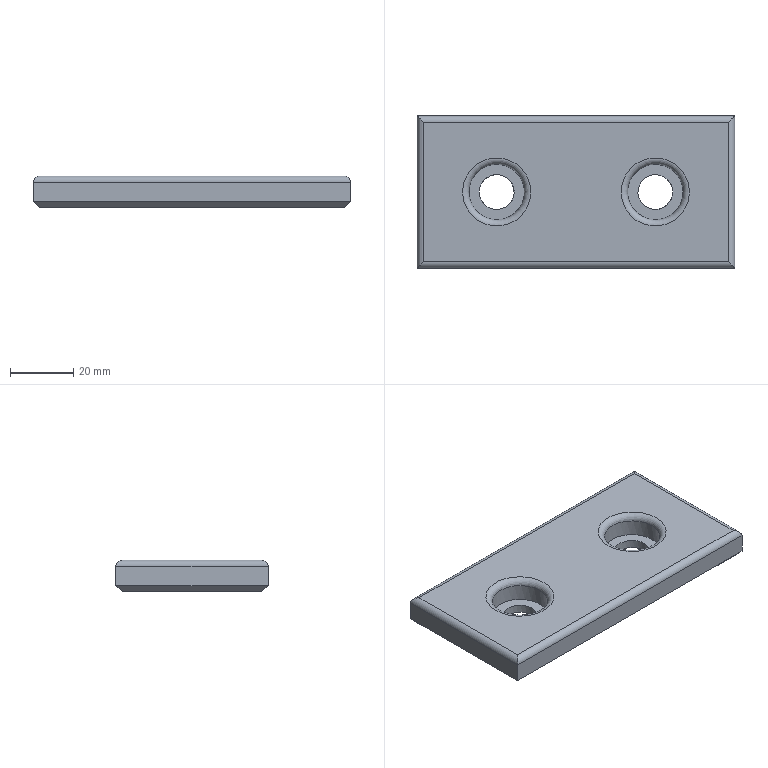Part | NX | features MAIN_BODY 2 | 1 solid | 22 faces | box 100 x 48 x 10 mm | volume 43044 mm3 | plane 12 | cylinder 8 | torus 2 | commonest cylinder face diameters 4 x4 11 x2 17.5 x2
STEP:
#1=CARTESIAN_POINT('',(267.,348.5,-80.));
#2=VERTEX_POINT('',#1);
#3=CARTESIAN_POINT('',(363.,348.5,-80.));
#4=VERTEX_POINT('',#3);
#5=CARTESIAN_POINT('',(365.,348.5,-80.));
#6=DIRECTION('',(-1.,0.,0.));
#7=VECTOR('',#6,1000.);
#8=LINE('',#5,#7);
#9=EDGE_CURVE('',#2,#4,#8,.F.);
#10=ORIENTED_EDGE('',*,*,#9,.F.);
#11=CARTESIAN_POINT('',(267.,304.5,-80.));
#12=VERTEX_POINT('',#11);
#13=CARTESIAN_POINT('',(267.,350.5,-80.));
#14=DIRECTION('',(0.,-1.,0.));
#15=VECTOR('',#14,1000.);
#16=LINE('',#13,#15);
#17=EDGE_CURVE('',#12,#2,#16,.F.);
#18=ORIENTED_EDGE('',*,*,#17,.F.);
#19=CARTESIAN_POINT('',(363.,304.5,-80.));
#20=VERTEX_POINT('',#19);
#21=CARTESIAN_POINT('',(365.,304.5,-80.));
#22=DIRECTION('',(1.,0.,0.));
#23=VECTOR('',#22,1000.);
#24=LINE('',#21,#23);
#25=EDGE_CURVE('',#20,#12,#24,.F.);
#26=ORIENTED_EDGE('',*,*,#25,.F.);
#27=CARTESIAN_POINT('',(363.,350.5,-80.));
#28=DIRECTION('',(0.,1.,0.));
#29=VECTOR('',#28,1000.);
#30=LINE('',#27,#29);
#31=EDGE_CURVE('',#4,#20,#30,.F.);
#32=ORIENTED_EDGE('',*,*,#31,.F.);
#33=EDGE_LOOP('',(#10,#18,#26,#32));
#34=FACE_BOUND('',#33,.T.);
#35=CARTESIAN_POINT('',(350.75,326.5,-80.));
#36=VERTEX_POINT('',#35);
#37=CARTESIAN_POINT('',(340.,326.5,-80.));
#38=DIRECTION('',(0.,0.,-1.));
#39=DIRECTION('',(1.,0.,0.));
#40=AXIS2_PLACEMENT_3D('',#37,#38,#39);
#41=CIRCLE('',#40,10.75);
#42=EDGE_CURVE('',#36,#36,#41,.F.);
#43=ORIENTED_EDGE('',*,*,#42,.F.);
#44=EDGE_LOOP('',(#43));
#45=FACE_BOUND('',#44,.T.);
#46=CARTESIAN_POINT('',(300.75,326.5,-80.));
#47=VERTEX_POINT('',#46);
#48=CARTESIAN_POINT('',(290.,326.5,-80.));
#49=DIRECTION('',(0.,0.,-1.));
#50=DIRECTION('',(1.,0.,0.));
#51=AXIS2_PLACEMENT_3D('',#48,#49,#50);
#52=CIRCLE('',#51,10.75);
#53=EDGE_CURVE('',#47,#47,#52,.F.);
#54=ORIENTED_EDGE('',*,*,#53,.F.);
#55=EDGE_LOOP('',(#54));
#56=FACE_BOUND('',#55,.T.);
#57=CARTESIAN_POINT('',(365.,350.5,-80.));
#58=DIRECTION('',(0.,0.,1.));
#59=DIRECTION('',(1.,0.,0.));
#60=AXIS2_PLACEMENT_3D('',#57,#58,#59);
#61=PLANE('',#60);
#62=ADVANCED_FACE('',(#34,#45,#56),#61,.T.);
#63=CARTESIAN_POINT('',(340.,321.,-90.));
#64=VERTEX_POINT('',#63);
#65=CARTESIAN_POINT('',(340.,326.5,-90.));
#66=DIRECTION('',(0.,0.,-1.));
#67=DIRECTION('',(0.,-1.,0.));
#68=AXIS2_PLACEMENT_3D('',#65,#66,#67);
#69=CIRCLE('',#68,5.5);
#70=EDGE_CURVE('',#64,#64,#69,.T.);
#71=ORIENTED_EDGE('',*,*,#70,.T.);
#72=EDGE_LOOP('',(#71));
#73=FACE_BOUND('',#72,.T.);
#74=CARTESIAN_POINT('',(345.5,326.5,-87.3));
#75=VERTEX_POINT('',#74);
#76=CARTESIAN_POINT('',(340.,326.5,-87.3));
#77=DIRECTION('',(0.,0.,-1.));
#78=DIRECTION('',(1.,0.,0.));
#79=AXIS2_PLACEMENT_3D('',#76,#77,#78);
#80=CIRCLE('',#79,5.5);
#81=EDGE_CURVE('',#75,#75,#80,.T.);
#82=ORIENTED_EDGE('',*,*,#81,.F.);
#83=EDGE_LOOP('',(#82));
#84=FACE_BOUND('',#83,.T.);
#85=CARTESIAN_POINT('',(340.,326.5,-70.));
#86=DIRECTION('',(0.,0.,-1.));
#87=DIRECTION('',(-1.,0.,0.));
#88=AXIS2_PLACEMENT_3D('',#85,#86,#87);
#89=CYLINDRICAL_SURFACE('',#88,5.5);
#90=ADVANCED_FACE('',(#73,#84),#89,.F.);
#91=CARTESIAN_POINT('',(267.,304.5,-90.));
#92=VERTEX_POINT('',#91);
#93=CARTESIAN_POINT('',(363.,304.5,-90.));
#94=VERTEX_POINT('',#93);
#95=CARTESIAN_POINT('',(365.,304.5,-90.));
#96=DIRECTION('',(1.,0.,0.));
#97=VECTOR('',#96,1000.);
#98=LINE('',#95,#97);
#99=EDGE_CURVE('',#92,#94,#98,.T.);
#100=ORIENTED_EDGE('',*,*,#99,.F.);
#101=CARTESIAN_POINT('',(267.,348.5,-90.));
#102=VERTEX_POINT('',#101);
#103=CARTESIAN_POINT('',(267.,302.5,-90.));
#104=DIRECTION('',(0.,-1.,0.));
#105=VECTOR('',#104,1000.);
#106=LINE('',#103,#105);
#107=EDGE_CURVE('',#102,#92,#106,.T.);
#108=ORIENTED_EDGE('',*,*,#107,.F.);
#109=CARTESIAN_POINT('',(363.,348.5,-90.));
#110=VERTEX_POINT('',#109);
#111=CARTESIAN_POINT('',(265.,348.5,-90.));
#112=DIRECTION('',(-1.,0.,0.));
#113=VECTOR('',#112,1000.);
#114=LINE('',#111,#113);
#115=EDGE_CURVE('',#110,#102,#114,.T.);
#116=ORIENTED_EDGE('',*,*,#115,.F.);
#117=CARTESIAN_POINT('',(363.,350.5,-90.));
#118=DIRECTION('',(0.,1.,0.));
#119=VECTOR('',#118,1000.);
#120=LINE('',#117,#119);
#121=EDGE_CURVE('',#94,#110,#120,.T.);
#122=ORIENTED_EDGE('',*,*,#121,.F.);
#123=EDGE_LOOP('',(#100,#108,#116,#122));
#124=FACE_BOUND('',#123,.T.);
#125=CARTESIAN_POINT('',(290.,321.,-90.));
#126=VERTEX_POINT('',#125);
#127=CARTESIAN_POINT('',(290.,326.5,-90.));
#128=DIRECTION('',(0.,0.,1.));
#129=DIRECTION('',(0.,-1.,0.));
#130=AXIS2_PLACEMENT_3D('',#127,#128,#129);
#131=CIRCLE('',#130,5.5);
#132=EDGE_CURVE('',#126,#126,#131,.T.);
#133=ORIENTED_EDGE('',*,*,#132,.T.);
#134=EDGE_LOOP('',(#133));
#135=FACE_BOUND('',#134,.T.);
#136=ORIENTED_EDGE('',*,*,#70,.F.);
#137=EDGE_LOOP('',(#136));
#138=FACE_BOUND('',#137,.T.);
#139=CARTESIAN_POINT('',(365.,350.5,-90.));
#140=DIRECTION('',(0.,0.,1.));
#141=DIRECTION('',(1.,0.,0.));
#142=AXIS2_PLACEMENT_3D('',#139,#140,#141);
#143=PLANE('',#142);
#144=ADVANCED_FACE('',(#124,#135,#138),#143,.F.);
#145=CARTESIAN_POINT('',(265.,350.5,-82.));
#146=VERTEX_POINT('',#145);
#147=CARTESIAN_POINT('',(265.,350.5,-88.));
#148=VERTEX_POINT('',#147);
#149=CARTESIAN_POINT('',(265.,350.5,-80.));
#150=DIRECTION('',(0.,0.,-1.));
#151=VECTOR('',#150,1000.);
#152=LINE('',#149,#151);
#153=EDGE_CURVE('',#146,#148,#152,.T.);
#154=ORIENTED_EDGE('',*,*,#153,.F.);
#155=CARTESIAN_POINT('',(365.,350.5,-82.));
#156=VERTEX_POINT('',#155);
#157=CARTESIAN_POINT('',(365.,350.5,-82.));
#158=DIRECTION('',(-1.,0.,0.));
#159=VECTOR('',#158,1000.);
#160=LINE('',#157,#159);
#161=EDGE_CURVE('',#156,#146,#160,.T.);
#162=ORIENTED_EDGE('',*,*,#161,.F.);
#163=CARTESIAN_POINT('',(365.,350.5,-88.));
#164=VERTEX_POINT('',#163);
#165=CARTESIAN_POINT('',(365.,350.5,-80.));
#166=DIRECTION('',(0.,0.,-1.));
#167=VECTOR('',#166,1000.);
#168=LINE('',#165,#167);
#169=EDGE_CURVE('',#156,#164,#168,.T.);
#170=ORIENTED_EDGE('',*,*,#169,.T.);
#171=CARTESIAN_POINT('',(365.,350.5,-88.));
#172=DIRECTION('',(1.,0.,0.));
#173=VECTOR('',#172,1000.);
#174=LINE('',#171,#173);
#175=EDGE_CURVE('',#148,#164,#174,.T.);
#176=ORIENTED_EDGE('',*,*,#175,.F.);
#177=EDGE_LOOP('',(#154,#162,#170,#176));
#178=FACE_BOUND('',#177,.T.);
#179=CARTESIAN_POINT('',(365.,350.5,-80.));
#180=DIRECTION('',(0.,1.,0.));
#181=DIRECTION('',(1.,0.,0.));
#182=AXIS2_PLACEMENT_3D('',#179,#180,#181);
#183=PLANE('',#182);
#184=ADVANCED_FACE('',(#178),#183,.T.);
#185=CARTESIAN_POINT('',(265.,302.5,-82.));
#186=VERTEX_POINT('',#185);
#187=CARTESIAN_POINT('',(265.,302.5,-88.));
#188=VERTEX_POINT('',#187);
#189=CARTESIAN_POINT('',(265.,302.5,-80.));
#190=DIRECTION('',(0.,0.,-1.));
#191=VECTOR('',#190,1000.);
#192=LINE('',#189,#191);
#193=EDGE_CURVE('',#186,#188,#192,.T.);
#194=ORIENTED_EDGE('',*,*,#193,.F.);
#195=CARTESIAN_POINT('',(265.,350.5,-82.));
#196=DIRECTION('',(0.,-1.,0.));
#197=VECTOR('',#196,1000.);
#198=LINE('',#195,#197);
#199=EDGE_CURVE('',#146,#186,#198,.T.);
#200=ORIENTED_EDGE('',*,*,#199,.F.);
#201=ORIENTED_EDGE('',*,*,#153,.T.);
#202=CARTESIAN_POINT('',(265.,350.5,-88.));
#203=DIRECTION('',(0.,1.,0.));
#204=VECTOR('',#203,1000.);
#205=LINE('',#202,#204);
#206=EDGE_CURVE('',#188,#148,#205,.T.);
#207=ORIENTED_EDGE('',*,*,#206,.F.);
#208=EDGE_LOOP('',(#194,#200,#201,#207));
#209=FACE_BOUND('',#208,.T.);
#210=CARTESIAN_POINT('',(265.,350.5,-80.));
#211=DIRECTION('',(-1.,0.,0.));
#212=DIRECTION('',(0.,0.,1.));
#213=AXIS2_PLACEMENT_3D('',#210,#211,#212);
#214=PLANE('',#213);
#215=ADVANCED_FACE('',(#209),#214,.T.);
#216=CARTESIAN_POINT('',(365.,302.5,-82.));
#217=VERTEX_POINT('',#216);
#218=CARTESIAN_POINT('',(365.,302.5,-88.));
#219=VERTEX_POINT('',#218);
#220=CARTESIAN_POINT('',(365.,302.5,-80.));
#221=DIRECTION('',(0.,0.,-1.));
#222=VECTOR('',#221,1000.);
#223=LINE('',#220,#222);
#224=EDGE_CURVE('',#217,#219,#223,.T.);
#225=ORIENTED_EDGE('',*,*,#224,.F.);
#226=CARTESIAN_POINT('',(265.,302.5,-82.));
#227=DIRECTION('',(1.,0.,0.));
#228=VECTOR('',#227,1000.);
#229=LINE('',#226,#228);
#230=EDGE_CURVE('',#186,#217,#229,.T.);
#231=ORIENTED_EDGE('',*,*,#230,.F.);
#232=ORIENTED_EDGE('',*,*,#193,.T.);
#233=CARTESIAN_POINT('',(265.,302.5,-88.));
#234=DIRECTION('',(-1.,0.,0.));
#235=VECTOR('',#234,1000.);
#236=LINE('',#233,#235);
#237=EDGE_CURVE('',#219,#188,#236,.T.);
#238=ORIENTED_EDGE('',*,*,#237,.F.);
#239=EDGE_LOOP('',(#225,#231,#232,#238));
#240=FACE_BOUND('',#239,.T.);
#241=CARTESIAN_POINT('',(265.,302.5,-80.));
#242=DIRECTION('',(0.,-1.,0.));
#243=DIRECTION('',(-1.,0.,0.));
#244=AXIS2_PLACEMENT_3D('',#241,#242,#243);
#245=PLANE('',#244);
#246=ADVANCED_FACE('',(#240),#245,.T.);
#247=ORIENTED_EDGE('',*,*,#169,.F.);
#248=CARTESIAN_POINT('',(365.,302.5,-82.));
#249=DIRECTION('',(0.,1.,0.));
#250=VECTOR('',#249,1000.);
#251=LINE('',#248,#250);
#252=EDGE_CURVE('',#217,#156,#251,.T.);
#253=ORIENTED_EDGE('',*,*,#252,.F.);
#254=ORIENTED_EDGE('',*,*,#224,.T.);
#255=CARTESIAN_POINT('',(365.,302.5,-88.));
#256=DIRECTION('',(0.,-1.,0.));
#257=VECTOR('',#256,1000.);
#258=LINE('',#255,#257);
#259=EDGE_CURVE('',#164,#219,#258,.T.);
#260=ORIENTED_EDGE('',*,*,#259,.F.);
#261=EDGE_LOOP('',(#247,#253,#254,#260));
#262=FACE_BOUND('',#261,.T.);
#263=CARTESIAN_POINT('',(365.,302.5,-80.));
#264=DIRECTION('',(1.,0.,0.));
#265=DIRECTION('',(0.,-1.,0.));
#266=AXIS2_PLACEMENT_3D('',#263,#264,#265);
#267=PLANE('',#266);
#268=ADVANCED_FACE('',(#262),#267,.T.);
#269=CARTESIAN_POINT('',(284.5,326.5,-87.3));
#270=VERTEX_POINT('',#269);
#271=CARTESIAN_POINT('',(290.,326.5,-87.3));
#272=DIRECTION('',(0.,0.,1.));
#273=DIRECTION('',(-1.,0.,0.));
#274=AXIS2_PLACEMENT_3D('',#271,#272,#273);
#275=CIRCLE('',#274,5.5);
#276=EDGE_CURVE('',#270,#270,#275,.F.);
#277=ORIENTED_EDGE('',*,*,#276,.F.);
#278=EDGE_LOOP('',(#277));
#279=FACE_BOUND('',#278,.T.);
#280=ORIENTED_EDGE('',*,*,#132,.F.);
#281=EDGE_LOOP('',(#280));
#282=FACE_BOUND('',#281,.T.);
#283=CARTESIAN_POINT('',(290.,326.5,-70.));
#284=DIRECTION('',(0.,0.,-1.));
#285=DIRECTION('',(-1.,0.,0.));
#286=AXIS2_PLACEMENT_3D('',#283,#284,#285);
#287=CYLINDRICAL_SURFACE('',#286,5.5);
#288=ADVANCED_FACE('',(#279,#282),#287,.F.);
#289=CARTESIAN_POINT('',(348.75,326.5,-82.));
#290=VERTEX_POINT('',#289);
#291=CARTESIAN_POINT('',(340.,326.5,-82.));
#292=DIRECTION('',(0.,0.,-1.));
#293=DIRECTION('',(1.,0.,0.));
#294=AXIS2_PLACEMENT_3D('',#291,#292,#293);
#295=CIRCLE('',#294,8.75);
#296=EDGE_CURVE('',#290,#290,#295,.T.);
#297=ORIENTED_EDGE('',*,*,#296,.F.);
#298=EDGE_LOOP('',(#297));
#299=FACE_BOUND('',#298,.T.);
#300=CARTESIAN_POINT('',(340.,317.75,-87.3));
#301=VERTEX_POINT('',#300);
#302=CARTESIAN_POINT('',(340.,326.5,-87.3));
#303=DIRECTION('',(0.,0.,-1.));
#304=DIRECTION('',(0.,-1.,0.));
#305=AXIS2_PLACEMENT_3D('',#302,#303,#304);
#306=CIRCLE('',#305,8.75);
#307=EDGE_CURVE('',#301,#301,#306,.T.);
#308=ORIENTED_EDGE('',*,*,#307,.T.);
#309=EDGE_LOOP('',(#308));
#310=FACE_BOUND('',#309,.T.);
#311=CARTESIAN_POINT('',(340.,326.5,-60.));
#312=DIRECTION('',(0.,0.,-1.));
#313=DIRECTION('',(-1.,0.,0.));
#314=AXIS2_PLACEMENT_3D('',#311,#312,#313);
#315=CYLINDRICAL_SURFACE('',#314,8.75);
#316=ADVANCED_FACE('',(#299,#310),#315,.F.);
#317=ORIENTED_EDGE('',*,*,#81,.T.);
#318=EDGE_LOOP('',(#317));
#319=FACE_BOUND('',#318,.T.);
#320=ORIENTED_EDGE('',*,*,#307,.F.);
#321=EDGE_LOOP('',(#320));
#322=FACE_BOUND('',#321,.T.);
#323=CARTESIAN_POINT('',(340.,326.5,-87.3));
#324=DIRECTION('',(0.,0.,1.));
#325=DIRECTION('',(1.,0.,0.));
#326=AXIS2_PLACEMENT_3D('',#323,#324,#325);
#327=PLANE('',#326);
#328=ADVANCED_FACE('',(#319,#322),#327,.T.);
#329=CARTESIAN_POINT('',(290.,317.75,-87.3));
#330=VERTEX_POINT('',#329);
#331=CARTESIAN_POINT('',(290.,326.5,-87.3));
#332=DIRECTION('',(0.,0.,1.));
#333=DIRECTION('',(0.,-1.,0.));
#334=AXIS2_PLACEMENT_3D('',#331,#332,#333);
#335=CIRCLE('',#334,8.75);
#336=EDGE_CURVE('',#330,#330,#335,.T.);
#337=ORIENTED_EDGE('',*,*,#336,.T.);
#338=EDGE_LOOP('',(#337));
#339=FACE_BOUND('',#338,.T.);
#340=ORIENTED_EDGE('',*,*,#276,.T.);
#341=EDGE_LOOP('',(#340));
#342=FACE_BOUND('',#341,.T.);
#343=CARTESIAN_POINT('',(290.,326.5,-87.3));
#344=DIRECTION('',(0.,0.,-1.));
#345=DIRECTION('',(-1.,0.,0.));
#346=AXIS2_PLACEMENT_3D('',#343,#344,#345);
#347=PLANE('',#346);
#348=ADVANCED_FACE('',(#339,#342),#347,.F.);
#349=CARTESIAN_POINT('',(298.75,326.5,-82.));
#350=VERTEX_POINT('',#349);
#351=CARTESIAN_POINT('',(290.,326.5,-82.));
#352=DIRECTION('',(0.,0.,-1.));
#353=DIRECTION('',(1.,0.,0.));
#354=AXIS2_PLACEMENT_3D('',#351,#352,#353);
#355=CIRCLE('',#354,8.75);
#356=EDGE_CURVE('',#350,#350,#355,.T.);
#357=ORIENTED_EDGE('',*,*,#356,.F.);
#358=EDGE_LOOP('',(#357));
#359=FACE_BOUND('',#358,.T.);
#360=ORIENTED_EDGE('',*,*,#336,.F.);
#361=EDGE_LOOP('',(#360));
#362=FACE_BOUND('',#361,.T.);
#363=CARTESIAN_POINT('',(290.,326.5,-60.));
#364=DIRECTION('',(0.,0.,-1.));
#365=DIRECTION('',(-1.,0.,0.));
#366=AXIS2_PLACEMENT_3D('',#363,#364,#365);
#367=CYLINDRICAL_SURFACE('',#366,8.75);
#368=ADVANCED_FACE('',(#359,#362),#367,.F.);
#369=CARTESIAN_POINT('',(267.,348.5,-82.));
#370=DIRECTION('',(0.7071,0.7071,0.));
#371=DIRECTION('',(0.7071,-0.7071,0.));
#372=AXIS2_PLACEMENT_3D('',#369,#370,#371);
#373=ELLIPSE('',#372,2.828,2.);
#374=EDGE_CURVE('',#2,#146,#373,.F.);
#375=ORIENTED_EDGE('',*,*,#374,.T.);
#376=ORIENTED_EDGE('',*,*,#199,.T.);
#377=CARTESIAN_POINT('',(267.,304.5,-82.));
#378=DIRECTION('',(-0.7071,0.7071,0.));
#379=DIRECTION('',(-0.7071,-0.7071,0.));
#380=AXIS2_PLACEMENT_3D('',#377,#378,#379);
#381=ELLIPSE('',#380,2.828,2.);
#382=EDGE_CURVE('',#186,#12,#381,.T.);
#383=ORIENTED_EDGE('',*,*,#382,.T.);
#384=ORIENTED_EDGE('',*,*,#17,.T.);
#385=EDGE_LOOP('',(#375,#376,#383,#384));
#386=FACE_BOUND('',#385,.T.);
#387=CARTESIAN_POINT('',(267.,350.5,-82.));
#388=DIRECTION('',(0.,-1.,0.));
#389=DIRECTION('',(-1.,0.,0.));
#390=AXIS2_PLACEMENT_3D('',#387,#388,#389);
#391=CYLINDRICAL_SURFACE('',#390,2.);
#392=ADVANCED_FACE('',(#386),#391,.T.);
#393=ORIENTED_EDGE('',*,*,#382,.F.);
#394=ORIENTED_EDGE('',*,*,#230,.T.);
#395=CARTESIAN_POINT('',(363.,304.5,-82.));
#396=DIRECTION('',(-0.7071,-0.7071,0.));
#397=DIRECTION('',(0.7071,-0.7071,0.));
#398=AXIS2_PLACEMENT_3D('',#395,#396,#397);
#399=ELLIPSE('',#398,2.828,2.);
#400=EDGE_CURVE('',#217,#20,#399,.T.);
#401=ORIENTED_EDGE('',*,*,#400,.T.);
#402=ORIENTED_EDGE('',*,*,#25,.T.);
#403=EDGE_LOOP('',(#393,#394,#401,#402));
#404=FACE_BOUND('',#403,.T.);
#405=CARTESIAN_POINT('',(265.,304.5,-82.));
#406=DIRECTION('',(1.,0.,0.));
#407=DIRECTION('',(0.,0.,-1.));
#408=AXIS2_PLACEMENT_3D('',#405,#406,#407);
#409=CYLINDRICAL_SURFACE('',#408,2.);
#410=ADVANCED_FACE('',(#404),#409,.T.);
#411=ORIENTED_EDGE('',*,*,#374,.F.);
#412=ORIENTED_EDGE('',*,*,#9,.T.);
#413=CARTESIAN_POINT('',(363.,348.5,-82.));
#414=DIRECTION('',(0.7071,-0.7071,0.));
#415=DIRECTION('',(-0.7071,-0.7071,0.));
#416=AXIS2_PLACEMENT_3D('',#413,#414,#415);
#417=ELLIPSE('',#416,2.828,2.);
#418=EDGE_CURVE('',#4,#156,#417,.F.);
#419=ORIENTED_EDGE('',*,*,#418,.T.);
#420=ORIENTED_EDGE('',*,*,#161,.T.);
#421=EDGE_LOOP('',(#411,#412,#419,#420));
#422=FACE_BOUND('',#421,.T.);
#423=CARTESIAN_POINT('',(365.,348.5,-82.));
#424=DIRECTION('',(-1.,0.,0.));
#425=DIRECTION('',(0.,1.,0.));
#426=AXIS2_PLACEMENT_3D('',#423,#424,#425);
#427=CYLINDRICAL_SURFACE('',#426,2.);
#428=ADVANCED_FACE('',(#422),#427,.T.);
#429=ORIENTED_EDGE('',*,*,#400,.F.);
#430=ORIENTED_EDGE('',*,*,#252,.T.);
#431=ORIENTED_EDGE('',*,*,#418,.F.);
#432=ORIENTED_EDGE('',*,*,#31,.T.);
#433=EDGE_LOOP('',(#429,#430,#431,#432));
#434=FACE_BOUND('',#433,.T.);
#435=CARTESIAN_POINT('',(363.,302.5,-82.));
#436=DIRECTION('',(0.,1.,0.));
#437=DIRECTION('',(1.,0.,0.));
#438=AXIS2_PLACEMENT_3D('',#435,#436,#437);
#439=CYLINDRICAL_SURFACE('',#438,2.);
#440=ADVANCED_FACE('',(#434),#439,.T.);
#441=ORIENTED_EDGE('',*,*,#296,.T.);
#442=EDGE_LOOP('',(#441));
#443=FACE_BOUND('',#442,.T.);
#444=ORIENTED_EDGE('',*,*,#42,.T.);
#445=EDGE_LOOP('',(#444));
#446=FACE_BOUND('',#445,.T.);
#447=CARTESIAN_POINT('',(340.,326.5,-82.));
#448=DIRECTION('',(0.,0.,1.));
#449=DIRECTION('',(1.,0.,0.));
#450=AXIS2_PLACEMENT_3D('',#447,#448,#449);
#451=TOROIDAL_SURFACE('',#450,10.75,2.);
#452=ADVANCED_FACE('',(#443,#446),#451,.T.);
#453=ORIENTED_EDGE('',*,*,#53,.T.);
#454=EDGE_LOOP('',(#453));
#455=FACE_BOUND('',#454,.T.);
#456=ORIENTED_EDGE('',*,*,#356,.T.);
#457=EDGE_LOOP('',(#456));
#458=FACE_BOUND('',#457,.T.);
#459=CARTESIAN_POINT('',(290.,326.5,-82.));
#460=DIRECTION('',(0.,0.,1.));
#461=DIRECTION('',(1.,0.,0.));
#462=AXIS2_PLACEMENT_3D('',#459,#460,#461);
#463=TOROIDAL_SURFACE('',#462,10.75,2.);
#464=ADVANCED_FACE('',(#455,#458),#463,.T.);
#465=CARTESIAN_POINT('',(266.333,349.167,-89.333));
#466=DIRECTION('',(-0.5774,0.5774,0.5774));
#467=VECTOR('',#466,1000.);
#468=LINE('',#465,#467);
#469=EDGE_CURVE('',#148,#102,#468,.F.);
#470=ORIENTED_EDGE('',*,*,#469,.T.);
#471=ORIENTED_EDGE('',*,*,#107,.T.);
#472=CARTESIAN_POINT('',(299.667,337.167,-122.667));
#473=DIRECTION('',(-0.5774,-0.5774,0.5774));
#474=VECTOR('',#473,1000.);
#475=LINE('',#472,#474);
#476=EDGE_CURVE('',#92,#188,#475,.T.);
#477=ORIENTED_EDGE('',*,*,#476,.T.);
#478=ORIENTED_EDGE('',*,*,#206,.T.);
#479=EDGE_LOOP('',(#470,#471,#477,#478));
#480=FACE_BOUND('',#479,.T.);
#481=CARTESIAN_POINT('',(267.,350.5,-90.));
#482=DIRECTION('',(-0.7071,0.,-0.7071));
#483=DIRECTION('',(-0.7071,0.,0.7071));
#484=AXIS2_PLACEMENT_3D('',#481,#482,#483);
#485=PLANE('',#484);
#486=ADVANCED_FACE('',(#480),#485,.T.);
#487=ORIENTED_EDGE('',*,*,#476,.F.);
#488=ORIENTED_EDGE('',*,*,#99,.T.);
#489=CARTESIAN_POINT('',(363.667,303.833,-89.333));
#490=DIRECTION('',(-0.5774,0.5774,-0.5774));
#491=VECTOR('',#490,1000.);
#492=LINE('',#489,#491);
#493=EDGE_CURVE('',#94,#219,#492,.F.);
#494=ORIENTED_EDGE('',*,*,#493,.T.);
#495=ORIENTED_EDGE('',*,*,#237,.T.);
#496=EDGE_LOOP('',(#487,#488,#494,#495));
#497=FACE_BOUND('',#496,.T.);
#498=CARTESIAN_POINT('',(365.,304.5,-90.));
#499=DIRECTION('',(0.,-0.7071,-0.7071));
#500=DIRECTION('',(0.,0.7071,-0.7071));
#501=AXIS2_PLACEMENT_3D('',#498,#499,#500);
#502=PLANE('',#501);
#503=ADVANCED_FACE('',(#497),#502,.T.);
#504=ORIENTED_EDGE('',*,*,#469,.F.);
#505=ORIENTED_EDGE('',*,*,#175,.T.);
#506=CARTESIAN_POINT('',(363.667,349.167,-89.333));
#507=DIRECTION('',(0.5774,0.5774,0.5774));
#508=VECTOR('',#507,1000.);
#509=LINE('',#506,#508);
#510=EDGE_CURVE('',#164,#110,#509,.F.);
#511=ORIENTED_EDGE('',*,*,#510,.T.);
#512=ORIENTED_EDGE('',*,*,#115,.T.);
#513=EDGE_LOOP('',(#504,#505,#511,#512));
#514=FACE_BOUND('',#513,.T.);
#515=CARTESIAN_POINT('',(365.,348.5,-90.));
#516=DIRECTION('',(0.,0.7071,-0.7071));
#517=DIRECTION('',(0.,0.7071,0.7071));
#518=AXIS2_PLACEMENT_3D('',#515,#516,#517);
#519=PLANE('',#518);
#520=ADVANCED_FACE('',(#514),#519,.T.);
#521=ORIENTED_EDGE('',*,*,#493,.F.);
#522=ORIENTED_EDGE('',*,*,#121,.T.);
#523=ORIENTED_EDGE('',*,*,#510,.F.);
#524=ORIENTED_EDGE('',*,*,#259,.T.);
#525=EDGE_LOOP('',(#521,#522,#523,#524));
#526=FACE_BOUND('',#525,.T.);
#527=CARTESIAN_POINT('',(363.,350.5,-90.));
#528=DIRECTION('',(0.7071,0.,-0.7071));
#529=DIRECTION('',(-0.7071,0.,-0.7071));
#530=AXIS2_PLACEMENT_3D('',#527,#528,#529);
#531=PLANE('',#530);
#532=ADVANCED_FACE('',(#526),#531,.T.);
#533=CLOSED_SHELL('',(#62,#90,#144,#184,#215,#246,#268,#288,#316,#328,#348,#368,#392,#410,#428,#440,#452,#464,#486,#503,#520,#532));
#534=MANIFOLD_SOLID_BREP('',#533);
#535=(LENGTH_UNIT()NAMED_UNIT(*)SI_UNIT(.MILLI.,.METRE.));
#536=UNCERTAINTY_MEASURE_WITH_UNIT(LENGTH_MEASURE(0.00001),#535,'','');
#537=(NAMED_UNIT(*)PLANE_ANGLE_UNIT()SI_UNIT($,.RADIAN.));
#538=(NAMED_UNIT(*)SI_UNIT($,.STERADIAN.)SOLID_ANGLE_UNIT());
#539=(GEOMETRIC_REPRESENTATION_CONTEXT(3)GLOBAL_UNCERTAINTY_ASSIGNED_CONTEXT((#536))GLOBAL_UNIT_ASSIGNED_CONTEXT((#535,#537,#538))REPRESENTATION_CONTEXT('',''));
#540=ADVANCED_BREP_SHAPE_REPRESENTATION('',(#534),#539);